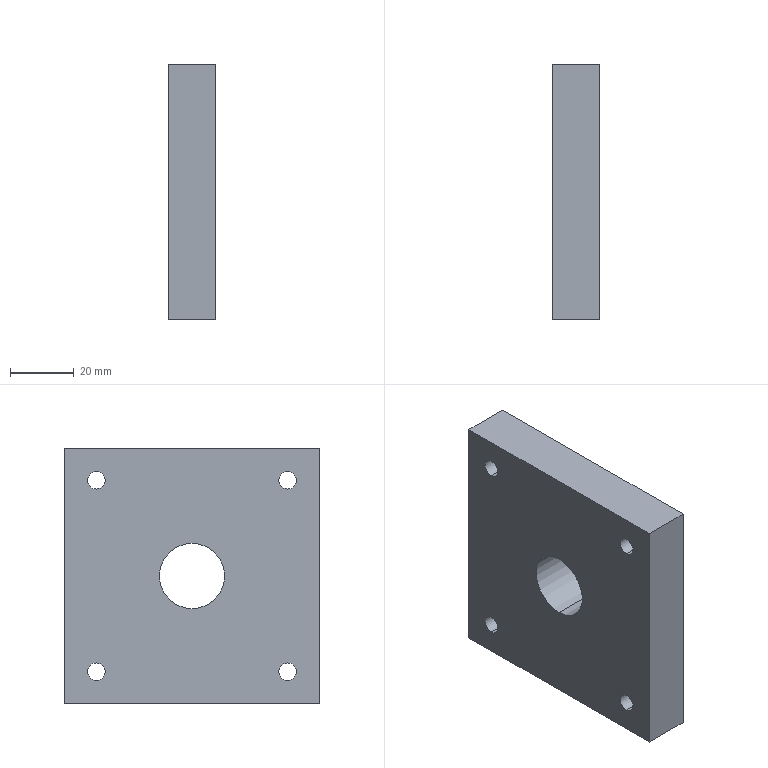Part | STEP file | 09-39 Cylinder top plate | 1 solid | 16 faces | box 15 x 80 x 80 mm | volume 89624 mm3 | cylinder 10 | plane 6 | commonest cylinder face diameters 5.5 x8 20.5 x2
STEP:
#1=CARTESIAN_POINT('',(0.,0.,0.));
#2=DIRECTION('',(0.,0.,1.));
#3=DIRECTION('',(1.,0.,0.));
#4=AXIS2_PLACEMENT_3D('',#1,#2,#3);
#5=CARTESIAN_POINT('',(0.,0.,-10.25));
#6=VERTEX_POINT('',#5);
#7=CARTESIAN_POINT('',(15.,0.,-10.25));
#8=VERTEX_POINT('',#7);
#9=CARTESIAN_POINT('',(0.,0.,-10.25));
#10=DIRECTION('',(1.,0.,0.));
#11=VECTOR('',#10,1.);
#12=LINE('',#9,#11);
#13=CARTESIAN_POINT('',(0.,0.,0.));
#14=DIRECTION('',(1.,0.,0.));
#15=DIRECTION('',(0.,0.,-1.));
#16=AXIS2_PLACEMENT_3D('',#13,#14,#15);
#17=CYLINDRICAL_SURFACE('',#16,10.25);
#18=CARTESIAN_POINT('',(6.283,0.));
#19=DIRECTION('',(0.,1.));
#20=VECTOR('',#19,1.);
#21=LINE('',#18,#20);
#22=(GEOMETRIC_REPRESENTATION_CONTEXT(2)PARAMETRIC_REPRESENTATION_CONTEXT()REPRESENTATION_CONTEXT('',''));
#23=DEFINITIONAL_REPRESENTATION('',(#21),#22);
#24=PCURVE('',#17,#23);
#25=CARTESIAN_POINT('',(0.,0.,0.));
#26=DIRECTION('',(1.,0.,0.));
#27=DIRECTION('',(0.,0.,-1.));
#28=AXIS2_PLACEMENT_3D('',#25,#26,#27);
#29=CYLINDRICAL_SURFACE('',#28,10.25);
#30=CARTESIAN_POINT('',(0.,0.));
#31=DIRECTION('',(0.,1.));
#32=VECTOR('',#31,1.);
#33=LINE('',#30,#32);
#34=(GEOMETRIC_REPRESENTATION_CONTEXT(2)PARAMETRIC_REPRESENTATION_CONTEXT()REPRESENTATION_CONTEXT('',''));
#35=DEFINITIONAL_REPRESENTATION('',(#33),#34);
#36=PCURVE('',#29,#35);
#37=SURFACE_CURVE('',#12,(#24,#36),.PCURVE_S1.);
#38=EDGE_CURVE('',#6,#8,#37,.T.);
#39=ORIENTED_EDGE('',*,*,#38,.T.);
#40=CARTESIAN_POINT('',(15.,0.,10.25));
#41=VERTEX_POINT('',#40);
#42=CARTESIAN_POINT('',(15.,0.,0.));
#43=DIRECTION('',(1.,0.,0.));
#44=DIRECTION('',(0.,0.,-1.));
#45=AXIS2_PLACEMENT_3D('',#42,#43,#44);
#46=CIRCLE('',#45,10.25);
#47=CARTESIAN_POINT('',(0.,15.));
#48=DIRECTION('',(1.,0.));
#49=VECTOR('',#48,1.);
#50=LINE('',#47,#49);
#51=(GEOMETRIC_REPRESENTATION_CONTEXT(2)PARAMETRIC_REPRESENTATION_CONTEXT()REPRESENTATION_CONTEXT('',''));
#52=DEFINITIONAL_REPRESENTATION('',(#50),#51);
#53=PCURVE('',#17,#52);
#54=CARTESIAN_POINT('',(15.,-40.,-40.));
#55=DIRECTION('',(-1.,0.,0.));
#56=DIRECTION('',(0.,0.,1.));
#57=AXIS2_PLACEMENT_3D('',#54,#55,#56);
#58=PLANE('',#57);
#59=CARTESIAN_POINT('',(29.75,40.));
#60=CARTESIAN_POINT('',(29.75,57.754));
#61=CARTESIAN_POINT('',(45.125,48.877));
#62=CARTESIAN_POINT('',(60.5,40.));
#63=CARTESIAN_POINT('',(45.125,31.123));
#64=CARTESIAN_POINT('',(29.75,22.246));
#65=CARTESIAN_POINT('',(29.75,40.));
#66=(BOUNDED_CURVE()B_SPLINE_CURVE(2,(#59,#60,#61,#62,#63,#64,#65),.UNSPECIFIED.,.T.,.F.)B_SPLINE_CURVE_WITH_KNOTS((1,2,2,2,2,1),(-2.094,0.,2.094,4.189,6.283,8.378),.UNSPECIFIED.)CURVE()GEOMETRIC_REPRESENTATION_ITEM()RATIONAL_B_SPLINE_CURVE((1.,0.5,1.,0.5,1.,0.5,1.))REPRESENTATION_ITEM(''));
#67=(GEOMETRIC_REPRESENTATION_CONTEXT(2)PARAMETRIC_REPRESENTATION_CONTEXT()REPRESENTATION_CONTEXT('',''));
#68=DEFINITIONAL_REPRESENTATION('',(#66),#67);
#69=PCURVE('',#58,#68);
#70=SURFACE_CURVE('',#46,(#53,#69),.PCURVE_S1.);
#71=EDGE_CURVE('',#41,#8,#70,.T.);
#72=ORIENTED_EDGE('',*,*,#71,.F.);
#73=CARTESIAN_POINT('',(0.,0.,10.25));
#74=VERTEX_POINT('',#73);
#75=CARTESIAN_POINT('',(0.,0.,10.25));
#76=DIRECTION('',(1.,0.,0.));
#77=VECTOR('',#76,1.);
#78=LINE('',#75,#77);
#79=CARTESIAN_POINT('',(3.142,0.));
#80=DIRECTION('',(0.,1.));
#81=VECTOR('',#80,1.);
#82=LINE('',#79,#81);
#83=(GEOMETRIC_REPRESENTATION_CONTEXT(2)PARAMETRIC_REPRESENTATION_CONTEXT()REPRESENTATION_CONTEXT('',''));
#84=DEFINITIONAL_REPRESENTATION('',(#82),#83);
#85=PCURVE('',#17,#84);
#86=CARTESIAN_POINT('',(3.142,0.));
#87=DIRECTION('',(0.,1.));
#88=VECTOR('',#87,1.);
#89=LINE('',#86,#88);
#90=(GEOMETRIC_REPRESENTATION_CONTEXT(2)PARAMETRIC_REPRESENTATION_CONTEXT()REPRESENTATION_CONTEXT('',''));
#91=DEFINITIONAL_REPRESENTATION('',(#89),#90);
#92=PCURVE('',#29,#91);
#93=SURFACE_CURVE('',#78,(#85,#92),.PCURVE_S1.);
#94=EDGE_CURVE('',#74,#41,#93,.T.);
#95=ORIENTED_EDGE('',*,*,#94,.F.);
#96=CARTESIAN_POINT('',(0.,0.,0.));
#97=DIRECTION('',(-1.,0.,0.));
#98=DIRECTION('',(0.,0.,-1.));
#99=AXIS2_PLACEMENT_3D('',#96,#97,#98);
#100=CIRCLE('',#99,10.25);
#101=CARTESIAN_POINT('',(6.283,0.));
#102=DIRECTION('',(-1.,0.));
#103=VECTOR('',#102,1.);
#104=LINE('',#101,#103);
#105=(GEOMETRIC_REPRESENTATION_CONTEXT(2)PARAMETRIC_REPRESENTATION_CONTEXT()REPRESENTATION_CONTEXT('',''));
#106=DEFINITIONAL_REPRESENTATION('',(#104),#105);
#107=PCURVE('',#17,#106);
#108=CARTESIAN_POINT('',(0.,-40.,-40.));
#109=DIRECTION('',(-1.,0.,0.));
#110=DIRECTION('',(0.,0.,1.));
#111=AXIS2_PLACEMENT_3D('',#108,#109,#110);
#112=PLANE('',#111);
#113=CARTESIAN_POINT('',(40.,40.));
#114=DIRECTION('',(-1.,0.));
#115=AXIS2_PLACEMENT_2D('',#113,#114);
#116=CIRCLE('',#115,10.25);
#117=(GEOMETRIC_REPRESENTATION_CONTEXT(2)PARAMETRIC_REPRESENTATION_CONTEXT()REPRESENTATION_CONTEXT('',''));
#118=DEFINITIONAL_REPRESENTATION('',(#116),#117);
#119=PCURVE('',#112,#118);
#120=SURFACE_CURVE('',#100,(#107,#119),.PCURVE_S1.);
#121=EDGE_CURVE('',#6,#74,#120,.T.);
#122=ORIENTED_EDGE('',*,*,#121,.F.);
#123=EDGE_LOOP('',(#39,#72,#95,#122));
#124=FACE_BOUND('',#123,.F.);
#125=ADVANCED_FACE('',(#124),#17,.F.);
#126=CARTESIAN_POINT('',(0.,30.,27.25));
#127=VERTEX_POINT('',#126);
#128=CARTESIAN_POINT('',(15.,30.,27.25));
#129=VERTEX_POINT('',#128);
#130=CARTESIAN_POINT('',(0.,30.,27.25));
#131=DIRECTION('',(1.,0.,0.));
#132=VECTOR('',#131,1.);
#133=LINE('',#130,#132);
#134=CARTESIAN_POINT('',(0.,30.,30.));
#135=DIRECTION('',(1.,0.,0.));
#136=DIRECTION('',(0.,0.,-1.));
#137=AXIS2_PLACEMENT_3D('',#134,#135,#136);
#138=CYLINDRICAL_SURFACE('',#137,2.75);
#139=CARTESIAN_POINT('',(6.283,0.));
#140=DIRECTION('',(0.,1.));
#141=VECTOR('',#140,1.);
#142=LINE('',#139,#141);
#143=(GEOMETRIC_REPRESENTATION_CONTEXT(2)PARAMETRIC_REPRESENTATION_CONTEXT()REPRESENTATION_CONTEXT('',''));
#144=DEFINITIONAL_REPRESENTATION('',(#142),#143);
#145=PCURVE('',#138,#144);
#146=CARTESIAN_POINT('',(0.,30.,30.));
#147=DIRECTION('',(1.,0.,0.));
#148=DIRECTION('',(0.,0.,-1.));
#149=AXIS2_PLACEMENT_3D('',#146,#147,#148);
#150=CYLINDRICAL_SURFACE('',#149,2.75);
#151=CARTESIAN_POINT('',(0.,0.));
#152=DIRECTION('',(0.,1.));
#153=VECTOR('',#152,1.);
#154=LINE('',#151,#153);
#155=(GEOMETRIC_REPRESENTATION_CONTEXT(2)PARAMETRIC_REPRESENTATION_CONTEXT()REPRESENTATION_CONTEXT('',''));
#156=DEFINITIONAL_REPRESENTATION('',(#154),#155);
#157=PCURVE('',#150,#156);
#158=SURFACE_CURVE('',#133,(#145,#157),.PCURVE_S1.);
#159=EDGE_CURVE('',#127,#129,#158,.T.);
#160=ORIENTED_EDGE('',*,*,#159,.T.);
#161=CARTESIAN_POINT('',(15.,30.,32.75));
#162=VERTEX_POINT('',#161);
#163=CARTESIAN_POINT('',(15.,30.,30.));
#164=DIRECTION('',(1.,0.,0.));
#165=DIRECTION('',(0.,0.,-1.));
#166=AXIS2_PLACEMENT_3D('',#163,#164,#165);
#167=CIRCLE('',#166,2.75);
#168=CARTESIAN_POINT('',(0.,15.));
#169=DIRECTION('',(1.,0.));
#170=VECTOR('',#169,1.);
#171=LINE('',#168,#170);
#172=(GEOMETRIC_REPRESENTATION_CONTEXT(2)PARAMETRIC_REPRESENTATION_CONTEXT()REPRESENTATION_CONTEXT('',''));
#173=DEFINITIONAL_REPRESENTATION('',(#171),#172);
#174=PCURVE('',#138,#173);
#175=CARTESIAN_POINT('',(67.25,70.));
#176=CARTESIAN_POINT('',(67.25,74.763));
#177=CARTESIAN_POINT('',(71.375,72.382));
#178=CARTESIAN_POINT('',(75.5,70.));
#179=CARTESIAN_POINT('',(71.375,67.618));
#180=CARTESIAN_POINT('',(67.25,65.237));
#181=CARTESIAN_POINT('',(67.25,70.));
#182=(BOUNDED_CURVE()B_SPLINE_CURVE(2,(#175,#176,#177,#178,#179,#180,#181),.UNSPECIFIED.,.T.,.F.)B_SPLINE_CURVE_WITH_KNOTS((1,2,2,2,2,1),(-2.094,0.,2.094,4.189,6.283,8.378),.UNSPECIFIED.)CURVE()GEOMETRIC_REPRESENTATION_ITEM()RATIONAL_B_SPLINE_CURVE((1.,0.5,1.,0.5,1.,0.5,1.))REPRESENTATION_ITEM(''));
#183=(GEOMETRIC_REPRESENTATION_CONTEXT(2)PARAMETRIC_REPRESENTATION_CONTEXT()REPRESENTATION_CONTEXT('',''));
#184=DEFINITIONAL_REPRESENTATION('',(#182),#183);
#185=PCURVE('',#58,#184);
#186=SURFACE_CURVE('',#167,(#174,#185),.PCURVE_S1.);
#187=EDGE_CURVE('',#162,#129,#186,.T.);
#188=ORIENTED_EDGE('',*,*,#187,.F.);
#189=CARTESIAN_POINT('',(0.,30.,32.75));
#190=VERTEX_POINT('',#189);
#191=CARTESIAN_POINT('',(0.,30.,32.75));
#192=DIRECTION('',(1.,0.,0.));
#193=VECTOR('',#192,1.);
#194=LINE('',#191,#193);
#195=CARTESIAN_POINT('',(3.142,0.));
#196=DIRECTION('',(0.,1.));
#197=VECTOR('',#196,1.);
#198=LINE('',#195,#197);
#199=(GEOMETRIC_REPRESENTATION_CONTEXT(2)PARAMETRIC_REPRESENTATION_CONTEXT()REPRESENTATION_CONTEXT('',''));
#200=DEFINITIONAL_REPRESENTATION('',(#198),#199);
#201=PCURVE('',#138,#200);
#202=CARTESIAN_POINT('',(3.142,0.));
#203=DIRECTION('',(0.,1.));
#204=VECTOR('',#203,1.);
#205=LINE('',#202,#204);
#206=(GEOMETRIC_REPRESENTATION_CONTEXT(2)PARAMETRIC_REPRESENTATION_CONTEXT()REPRESENTATION_CONTEXT('',''));
#207=DEFINITIONAL_REPRESENTATION('',(#205),#206);
#208=PCURVE('',#150,#207);
#209=SURFACE_CURVE('',#194,(#201,#208),.PCURVE_S1.);
#210=EDGE_CURVE('',#190,#162,#209,.T.);
#211=ORIENTED_EDGE('',*,*,#210,.F.);
#212=CARTESIAN_POINT('',(0.,30.,30.));
#213=DIRECTION('',(1.,0.,0.));
#214=DIRECTION('',(0.,0.,-1.));
#215=AXIS2_PLACEMENT_3D('',#212,#213,#214);
#216=CIRCLE('',#215,2.75);
#217=CARTESIAN_POINT('',(0.,0.));
#218=DIRECTION('',(1.,0.));
#219=VECTOR('',#218,1.);
#220=LINE('',#217,#219);
#221=(GEOMETRIC_REPRESENTATION_CONTEXT(2)PARAMETRIC_REPRESENTATION_CONTEXT()REPRESENTATION_CONTEXT('',''));
#222=DEFINITIONAL_REPRESENTATION('',(#220),#221);
#223=PCURVE('',#138,#222);
#224=CARTESIAN_POINT('',(67.25,70.));
#225=CARTESIAN_POINT('',(67.25,74.763));
#226=CARTESIAN_POINT('',(71.375,72.382));
#227=CARTESIAN_POINT('',(75.5,70.));
#228=CARTESIAN_POINT('',(71.375,67.618));
#229=CARTESIAN_POINT('',(67.25,65.237));
#230=CARTESIAN_POINT('',(67.25,70.));
#231=(BOUNDED_CURVE()B_SPLINE_CURVE(2,(#224,#225,#226,#227,#228,#229,#230),.UNSPECIFIED.,.T.,.F.)B_SPLINE_CURVE_WITH_KNOTS((1,2,2,2,2,1),(-2.094,0.,2.094,4.189,6.283,8.378),.UNSPECIFIED.)CURVE()GEOMETRIC_REPRESENTATION_ITEM()RATIONAL_B_SPLINE_CURVE((1.,0.5,1.,0.5,1.,0.5,1.))REPRESENTATION_ITEM(''));
#232=(GEOMETRIC_REPRESENTATION_CONTEXT(2)PARAMETRIC_REPRESENTATION_CONTEXT()REPRESENTATION_CONTEXT('',''));
#233=DEFINITIONAL_REPRESENTATION('',(#231),#232);
#234=PCURVE('',#112,#233);
#235=SURFACE_CURVE('',#216,(#223,#234),.PCURVE_S1.);
#236=EDGE_CURVE('',#190,#127,#235,.T.);
#237=ORIENTED_EDGE('',*,*,#236,.T.);
#238=EDGE_LOOP('',(#160,#188,#211,#237));
#239=FACE_BOUND('',#238,.F.);
#240=ADVANCED_FACE('',(#239),#138,.F.);
#241=CARTESIAN_POINT('',(0.,30.,-32.75));
#242=VERTEX_POINT('',#241);
#243=CARTESIAN_POINT('',(15.,30.,-32.75));
#244=VERTEX_POINT('',#243);
#245=CARTESIAN_POINT('',(0.,30.,-32.75));
#246=DIRECTION('',(1.,0.,0.));
#247=VECTOR('',#246,1.);
#248=LINE('',#245,#247);
#249=CARTESIAN_POINT('',(0.,30.,-30.));
#250=DIRECTION('',(1.,0.,0.));
#251=DIRECTION('',(0.,0.,-1.));
#252=AXIS2_PLACEMENT_3D('',#249,#250,#251);
#253=CYLINDRICAL_SURFACE('',#252,2.75);
#254=CARTESIAN_POINT('',(6.283,0.));
#255=DIRECTION('',(0.,1.));
#256=VECTOR('',#255,1.);
#257=LINE('',#254,#256);
#258=(GEOMETRIC_REPRESENTATION_CONTEXT(2)PARAMETRIC_REPRESENTATION_CONTEXT()REPRESENTATION_CONTEXT('',''));
#259=DEFINITIONAL_REPRESENTATION('',(#257),#258);
#260=PCURVE('',#253,#259);
#261=CARTESIAN_POINT('',(0.,30.,-30.));
#262=DIRECTION('',(1.,0.,0.));
#263=DIRECTION('',(0.,0.,-1.));
#264=AXIS2_PLACEMENT_3D('',#261,#262,#263);
#265=CYLINDRICAL_SURFACE('',#264,2.75);
#266=CARTESIAN_POINT('',(0.,0.));
#267=DIRECTION('',(0.,1.));
#268=VECTOR('',#267,1.);
#269=LINE('',#266,#268);
#270=(GEOMETRIC_REPRESENTATION_CONTEXT(2)PARAMETRIC_REPRESENTATION_CONTEXT()REPRESENTATION_CONTEXT('',''));
#271=DEFINITIONAL_REPRESENTATION('',(#269),#270);
#272=PCURVE('',#265,#271);
#273=SURFACE_CURVE('',#248,(#260,#272),.PCURVE_S1.);
#274=EDGE_CURVE('',#242,#244,#273,.T.);
#275=ORIENTED_EDGE('',*,*,#274,.T.);
#276=CARTESIAN_POINT('',(15.,30.,-27.25));
#277=VERTEX_POINT('',#276);
#278=CARTESIAN_POINT('',(15.,30.,-30.));
#279=DIRECTION('',(1.,0.,0.));
#280=DIRECTION('',(0.,0.,-1.));
#281=AXIS2_PLACEMENT_3D('',#278,#279,#280);
#282=CIRCLE('',#281,2.75);
#283=CARTESIAN_POINT('',(0.,15.));
#284=DIRECTION('',(1.,0.));
#285=VECTOR('',#284,1.);
#286=LINE('',#283,#285);
#287=(GEOMETRIC_REPRESENTATION_CONTEXT(2)PARAMETRIC_REPRESENTATION_CONTEXT()REPRESENTATION_CONTEXT('',''));
#288=DEFINITIONAL_REPRESENTATION('',(#286),#287);
#289=PCURVE('',#253,#288);
#290=CARTESIAN_POINT('',(7.25,70.));
#291=CARTESIAN_POINT('',(7.25,74.763));
#292=CARTESIAN_POINT('',(11.375,72.382));
#293=CARTESIAN_POINT('',(15.5,70.));
#294=CARTESIAN_POINT('',(11.375,67.618));
#295=CARTESIAN_POINT('',(7.25,65.237));
#296=CARTESIAN_POINT('',(7.25,70.));
#297=(BOUNDED_CURVE()B_SPLINE_CURVE(2,(#290,#291,#292,#293,#294,#295,#296),.UNSPECIFIED.,.T.,.F.)B_SPLINE_CURVE_WITH_KNOTS((1,2,2,2,2,1),(-2.094,0.,2.094,4.189,6.283,8.378),.UNSPECIFIED.)CURVE()GEOMETRIC_REPRESENTATION_ITEM()RATIONAL_B_SPLINE_CURVE((1.,0.5,1.,0.5,1.,0.5,1.))REPRESENTATION_ITEM(''));
#298=(GEOMETRIC_REPRESENTATION_CONTEXT(2)PARAMETRIC_REPRESENTATION_CONTEXT()REPRESENTATION_CONTEXT('',''));
#299=DEFINITIONAL_REPRESENTATION('',(#297),#298);
#300=PCURVE('',#58,#299);
#301=SURFACE_CURVE('',#282,(#289,#300),.PCURVE_S1.);
#302=EDGE_CURVE('',#277,#244,#301,.T.);
#303=ORIENTED_EDGE('',*,*,#302,.F.);
#304=CARTESIAN_POINT('',(0.,30.,-27.25));
#305=VERTEX_POINT('',#304);
#306=CARTESIAN_POINT('',(0.,30.,-27.25));
#307=DIRECTION('',(1.,0.,0.));
#308=VECTOR('',#307,1.);
#309=LINE('',#306,#308);
#310=CARTESIAN_POINT('',(3.142,0.));
#311=DIRECTION('',(0.,1.));
#312=VECTOR('',#311,1.);
#313=LINE('',#310,#312);
#314=(GEOMETRIC_REPRESENTATION_CONTEXT(2)PARAMETRIC_REPRESENTATION_CONTEXT()REPRESENTATION_CONTEXT('',''));
#315=DEFINITIONAL_REPRESENTATION('',(#313),#314);
#316=PCURVE('',#253,#315);
#317=CARTESIAN_POINT('',(3.142,0.));
#318=DIRECTION('',(0.,1.));
#319=VECTOR('',#318,1.);
#320=LINE('',#317,#319);
#321=(GEOMETRIC_REPRESENTATION_CONTEXT(2)PARAMETRIC_REPRESENTATION_CONTEXT()REPRESENTATION_CONTEXT('',''));
#322=DEFINITIONAL_REPRESENTATION('',(#320),#321);
#323=PCURVE('',#265,#322);
#324=SURFACE_CURVE('',#309,(#316,#323),.PCURVE_S1.);
#325=EDGE_CURVE('',#305,#277,#324,.T.);
#326=ORIENTED_EDGE('',*,*,#325,.F.);
#327=CARTESIAN_POINT('',(0.,30.,-30.));
#328=DIRECTION('',(1.,0.,0.));
#329=DIRECTION('',(0.,0.,-1.));
#330=AXIS2_PLACEMENT_3D('',#327,#328,#329);
#331=CIRCLE('',#330,2.75);
#332=CARTESIAN_POINT('',(0.,0.));
#333=DIRECTION('',(1.,0.));
#334=VECTOR('',#333,1.);
#335=LINE('',#332,#334);
#336=(GEOMETRIC_REPRESENTATION_CONTEXT(2)PARAMETRIC_REPRESENTATION_CONTEXT()REPRESENTATION_CONTEXT('',''));
#337=DEFINITIONAL_REPRESENTATION('',(#335),#336);
#338=PCURVE('',#253,#337);
#339=CARTESIAN_POINT('',(7.25,70.));
#340=CARTESIAN_POINT('',(7.25,74.763));
#341=CARTESIAN_POINT('',(11.375,72.382));
#342=CARTESIAN_POINT('',(15.5,70.));
#343=CARTESIAN_POINT('',(11.375,67.618));
#344=CARTESIAN_POINT('',(7.25,65.237));
#345=CARTESIAN_POINT('',(7.25,70.));
#346=(BOUNDED_CURVE()B_SPLINE_CURVE(2,(#339,#340,#341,#342,#343,#344,#345),.UNSPECIFIED.,.T.,.F.)B_SPLINE_CURVE_WITH_KNOTS((1,2,2,2,2,1),(-2.094,0.,2.094,4.189,6.283,8.378),.UNSPECIFIED.)CURVE()GEOMETRIC_REPRESENTATION_ITEM()RATIONAL_B_SPLINE_CURVE((1.,0.5,1.,0.5,1.,0.5,1.))REPRESENTATION_ITEM(''));
#347=(GEOMETRIC_REPRESENTATION_CONTEXT(2)PARAMETRIC_REPRESENTATION_CONTEXT()REPRESENTATION_CONTEXT('',''));
#348=DEFINITIONAL_REPRESENTATION('',(#346),#347);
#349=PCURVE('',#112,#348);
#350=SURFACE_CURVE('',#331,(#338,#349),.PCURVE_S1.);
#351=EDGE_CURVE('',#305,#242,#350,.T.);
#352=ORIENTED_EDGE('',*,*,#351,.T.);
#353=EDGE_LOOP('',(#275,#303,#326,#352));
#354=FACE_BOUND('',#353,.F.);
#355=ADVANCED_FACE('',(#354),#253,.F.);
#356=CARTESIAN_POINT('',(0.,-30.,-32.75));
#357=VERTEX_POINT('',#356);
#358=CARTESIAN_POINT('',(15.,-30.,-32.75));
#359=VERTEX_POINT('',#358);
#360=CARTESIAN_POINT('',(0.,-30.,-32.75));
#361=DIRECTION('',(1.,0.,0.));
#362=VECTOR('',#361,1.);
#363=LINE('',#360,#362);
#364=CARTESIAN_POINT('',(0.,-30.,-30.));
#365=DIRECTION('',(1.,0.,0.));
#366=DIRECTION('',(0.,0.,-1.));
#367=AXIS2_PLACEMENT_3D('',#364,#365,#366);
#368=CYLINDRICAL_SURFACE('',#367,2.75);
#369=CARTESIAN_POINT('',(6.283,0.));
#370=DIRECTION('',(0.,1.));
#371=VECTOR('',#370,1.);
#372=LINE('',#369,#371);
#373=(GEOMETRIC_REPRESENTATION_CONTEXT(2)PARAMETRIC_REPRESENTATION_CONTEXT()REPRESENTATION_CONTEXT('',''));
#374=DEFINITIONAL_REPRESENTATION('',(#372),#373);
#375=PCURVE('',#368,#374);
#376=CARTESIAN_POINT('',(0.,-30.,-30.));
#377=DIRECTION('',(1.,0.,0.));
#378=DIRECTION('',(0.,0.,-1.));
#379=AXIS2_PLACEMENT_3D('',#376,#377,#378);
#380=CYLINDRICAL_SURFACE('',#379,2.75);
#381=CARTESIAN_POINT('',(0.,0.));
#382=DIRECTION('',(0.,1.));
#383=VECTOR('',#382,1.);
#384=LINE('',#381,#383);
#385=(GEOMETRIC_REPRESENTATION_CONTEXT(2)PARAMETRIC_REPRESENTATION_CONTEXT()REPRESENTATION_CONTEXT('',''));
#386=DEFINITIONAL_REPRESENTATION('',(#384),#385);
#387=PCURVE('',#380,#386);
#388=SURFACE_CURVE('',#363,(#375,#387),.PCURVE_S1.);
#389=EDGE_CURVE('',#357,#359,#388,.T.);
#390=ORIENTED_EDGE('',*,*,#389,.T.);
#391=CARTESIAN_POINT('',(15.,-30.,-27.25));
#392=VERTEX_POINT('',#391);
#393=CARTESIAN_POINT('',(15.,-30.,-30.));
#394=DIRECTION('',(1.,0.,0.));
#395=DIRECTION('',(0.,0.,-1.));
#396=AXIS2_PLACEMENT_3D('',#393,#394,#395);
#397=CIRCLE('',#396,2.75);
#398=CARTESIAN_POINT('',(0.,15.));
#399=DIRECTION('',(1.,0.));
#400=VECTOR('',#399,1.);
#401=LINE('',#398,#400);
#402=(GEOMETRIC_REPRESENTATION_CONTEXT(2)PARAMETRIC_REPRESENTATION_CONTEXT()REPRESENTATION_CONTEXT('',''));
#403=DEFINITIONAL_REPRESENTATION('',(#401),#402);
#404=PCURVE('',#368,#403);
#405=CARTESIAN_POINT('',(7.25,10.));
#406=CARTESIAN_POINT('',(7.25,14.763));
#407=CARTESIAN_POINT('',(11.375,12.382));
#408=CARTESIAN_POINT('',(15.5,10.));
#409=CARTESIAN_POINT('',(11.375,7.618));
#410=CARTESIAN_POINT('',(7.25,5.237));
#411=CARTESIAN_POINT('',(7.25,10.));
#412=(BOUNDED_CURVE()B_SPLINE_CURVE(2,(#405,#406,#407,#408,#409,#410,#411),.UNSPECIFIED.,.T.,.F.)B_SPLINE_CURVE_WITH_KNOTS((1,2,2,2,2,1),(-2.094,0.,2.094,4.189,6.283,8.378),.UNSPECIFIED.)CURVE()GEOMETRIC_REPRESENTATION_ITEM()RATIONAL_B_SPLINE_CURVE((1.,0.5,1.,0.5,1.,0.5,1.))REPRESENTATION_ITEM(''));
#413=(GEOMETRIC_REPRESENTATION_CONTEXT(2)PARAMETRIC_REPRESENTATION_CONTEXT()REPRESENTATION_CONTEXT('',''));
#414=DEFINITIONAL_REPRESENTATION('',(#412),#413);
#415=PCURVE('',#58,#414);
#416=SURFACE_CURVE('',#397,(#404,#415),.PCURVE_S1.);
#417=EDGE_CURVE('',#392,#359,#416,.T.);
#418=ORIENTED_EDGE('',*,*,#417,.F.);
#419=CARTESIAN_POINT('',(0.,-30.,-27.25));
#420=VERTEX_POINT('',#419);
#421=CARTESIAN_POINT('',(0.,-30.,-27.25));
#422=DIRECTION('',(1.,0.,0.));
#423=VECTOR('',#422,1.);
#424=LINE('',#421,#423);
#425=CARTESIAN_POINT('',(3.142,0.));
#426=DIRECTION('',(0.,1.));
#427=VECTOR('',#426,1.);
#428=LINE('',#425,#427);
#429=(GEOMETRIC_REPRESENTATION_CONTEXT(2)PARAMETRIC_REPRESENTATION_CONTEXT()REPRESENTATION_CONTEXT('',''));
#430=DEFINITIONAL_REPRESENTATION('',(#428),#429);
#431=PCURVE('',#368,#430);
#432=CARTESIAN_POINT('',(3.142,0.));
#433=DIRECTION('',(0.,1.));
#434=VECTOR('',#433,1.);
#435=LINE('',#432,#434);
#436=(GEOMETRIC_REPRESENTATION_CONTEXT(2)PARAMETRIC_REPRESENTATION_CONTEXT()REPRESENTATION_CONTEXT('',''));
#437=DEFINITIONAL_REPRESENTATION('',(#435),#436);
#438=PCURVE('',#380,#437);
#439=SURFACE_CURVE('',#424,(#431,#438),.PCURVE_S1.);
#440=EDGE_CURVE('',#420,#392,#439,.T.);
#441=ORIENTED_EDGE('',*,*,#440,.F.);
#442=CARTESIAN_POINT('',(0.,-30.,-30.));
#443=DIRECTION('',(1.,0.,0.));
#444=DIRECTION('',(0.,0.,-1.));
#445=AXIS2_PLACEMENT_3D('',#442,#443,#444);
#446=CIRCLE('',#445,2.75);
#447=CARTESIAN_POINT('',(0.,0.));
#448=DIRECTION('',(1.,0.));
#449=VECTOR('',#448,1.);
#450=LINE('',#447,#449);
#451=(GEOMETRIC_REPRESENTATION_CONTEXT(2)PARAMETRIC_REPRESENTATION_CONTEXT()REPRESENTATION_CONTEXT('',''));
#452=DEFINITIONAL_REPRESENTATION('',(#450),#451);
#453=PCURVE('',#368,#452);
#454=CARTESIAN_POINT('',(7.25,10.));
#455=CARTESIAN_POINT('',(7.25,14.763));
#456=CARTESIAN_POINT('',(11.375,12.382));
#457=CARTESIAN_POINT('',(15.5,10.));
#458=CARTESIAN_POINT('',(11.375,7.618));
#459=CARTESIAN_POINT('',(7.25,5.237));
#460=CARTESIAN_POINT('',(7.25,10.));
#461=(BOUNDED_CURVE()B_SPLINE_CURVE(2,(#454,#455,#456,#457,#458,#459,#460),.UNSPECIFIED.,.T.,.F.)B_SPLINE_CURVE_WITH_KNOTS((1,2,2,2,2,1),(-2.094,0.,2.094,4.189,6.283,8.378),.UNSPECIFIED.)CURVE()GEOMETRIC_REPRESENTATION_ITEM()RATIONAL_B_SPLINE_CURVE((1.,0.5,1.,0.5,1.,0.5,1.))REPRESENTATION_ITEM(''));
#462=(GEOMETRIC_REPRESENTATION_CONTEXT(2)PARAMETRIC_REPRESENTATION_CONTEXT()REPRESENTATION_CONTEXT('',''));
#463=DEFINITIONAL_REPRESENTATION('',(#461),#462);
#464=PCURVE('',#112,#463);
#465=SURFACE_CURVE('',#446,(#453,#464),.PCURVE_S1.);
#466=EDGE_CURVE('',#420,#357,#465,.T.);
#467=ORIENTED_EDGE('',*,*,#466,.T.);
#468=EDGE_LOOP('',(#390,#418,#441,#467));
#469=FACE_BOUND('',#468,.F.);
#470=ADVANCED_FACE('',(#469),#368,.F.);
#471=CARTESIAN_POINT('',(0.,-30.,27.25));
#472=VERTEX_POINT('',#471);
#473=CARTESIAN_POINT('',(15.,-30.,27.25));
#474=VERTEX_POINT('',#473);
#475=CARTESIAN_POINT('',(0.,-30.,27.25));
#476=DIRECTION('',(1.,0.,0.));
#477=VECTOR('',#476,1.);
#478=LINE('',#475,#477);
#479=CARTESIAN_POINT('',(0.,-30.,30.));
#480=DIRECTION('',(1.,0.,0.));
#481=DIRECTION('',(0.,0.,-1.));
#482=AXIS2_PLACEMENT_3D('',#479,#480,#481);
#483=CYLINDRICAL_SURFACE('',#482,2.75);
#484=CARTESIAN_POINT('',(6.283,0.));
#485=DIRECTION('',(0.,1.));
#486=VECTOR('',#485,1.);
#487=LINE('',#484,#486);
#488=(GEOMETRIC_REPRESENTATION_CONTEXT(2)PARAMETRIC_REPRESENTATION_CONTEXT()REPRESENTATION_CONTEXT('',''));
#489=DEFINITIONAL_REPRESENTATION('',(#487),#488);
#490=PCURVE('',#483,#489);
#491=CARTESIAN_POINT('',(0.,-30.,30.));
#492=DIRECTION('',(1.,0.,0.));
#493=DIRECTION('',(0.,0.,-1.));
#494=AXIS2_PLACEMENT_3D('',#491,#492,#493);
#495=CYLINDRICAL_SURFACE('',#494,2.75);
#496=CARTESIAN_POINT('',(0.,0.));
#497=DIRECTION('',(0.,1.));
#498=VECTOR('',#497,1.);
#499=LINE('',#496,#498);
#500=(GEOMETRIC_REPRESENTATION_CONTEXT(2)PARAMETRIC_REPRESENTATION_CONTEXT()REPRESENTATION_CONTEXT('',''));
#501=DEFINITIONAL_REPRESENTATION('',(#499),#500);
#502=PCURVE('',#495,#501);
#503=SURFACE_CURVE('',#478,(#490,#502),.PCURVE_S1.);
#504=EDGE_CURVE('',#472,#474,#503,.T.);
#505=ORIENTED_EDGE('',*,*,#504,.T.);
#506=CARTESIAN_POINT('',(15.,-30.,32.75));
#507=VERTEX_POINT('',#506);
#508=CARTESIAN_POINT('',(15.,-30.,30.));
#509=DIRECTION('',(1.,0.,0.));
#510=DIRECTION('',(0.,0.,-1.));
#511=AXIS2_PLACEMENT_3D('',#508,#509,#510);
#512=CIRCLE('',#511,2.75);
#513=CARTESIAN_POINT('',(0.,15.));
#514=DIRECTION('',(1.,0.));
#515=VECTOR('',#514,1.);
#516=LINE('',#513,#515);
#517=(GEOMETRIC_REPRESENTATION_CONTEXT(2)PARAMETRIC_REPRESENTATION_CONTEXT()REPRESENTATION_CONTEXT('',''));
#518=DEFINITIONAL_REPRESENTATION('',(#516),#517);
#519=PCURVE('',#483,#518);
#520=CARTESIAN_POINT('',(67.25,10.));
#521=CARTESIAN_POINT('',(67.25,14.763));
#522=CARTESIAN_POINT('',(71.375,12.382));
#523=CARTESIAN_POINT('',(75.5,10.));
#524=CARTESIAN_POINT('',(71.375,7.618));
#525=CARTESIAN_POINT('',(67.25,5.237));
#526=CARTESIAN_POINT('',(67.25,10.));
#527=(BOUNDED_CURVE()B_SPLINE_CURVE(2,(#520,#521,#522,#523,#524,#525,#526),.UNSPECIFIED.,.T.,.F.)B_SPLINE_CURVE_WITH_KNOTS((1,2,2,2,2,1),(-2.094,0.,2.094,4.189,6.283,8.378),.UNSPECIFIED.)CURVE()GEOMETRIC_REPRESENTATION_ITEM()RATIONAL_B_SPLINE_CURVE((1.,0.5,1.,0.5,1.,0.5,1.))REPRESENTATION_ITEM(''));
#528=(GEOMETRIC_REPRESENTATION_CONTEXT(2)PARAMETRIC_REPRESENTATION_CONTEXT()REPRESENTATION_CONTEXT('',''));
#529=DEFINITIONAL_REPRESENTATION('',(#527),#528);
#530=PCURVE('',#58,#529);
#531=SURFACE_CURVE('',#512,(#519,#530),.PCURVE_S1.);
#532=EDGE_CURVE('',#507,#474,#531,.T.);
#533=ORIENTED_EDGE('',*,*,#532,.F.);
#534=CARTESIAN_POINT('',(0.,-30.,32.75));
#535=VERTEX_POINT('',#534);
#536=CARTESIAN_POINT('',(0.,-30.,32.75));
#537=DIRECTION('',(1.,0.,0.));
#538=VECTOR('',#537,1.);
#539=LINE('',#536,#538);
#540=CARTESIAN_POINT('',(3.142,0.));
#541=DIRECTION('',(0.,1.));
#542=VECTOR('',#541,1.);
#543=LINE('',#540,#542);
#544=(GEOMETRIC_REPRESENTATION_CONTEXT(2)PARAMETRIC_REPRESENTATION_CONTEXT()REPRESENTATION_CONTEXT('',''));
#545=DEFINITIONAL_REPRESENTATION('',(#543),#544);
#546=PCURVE('',#483,#545);
#547=CARTESIAN_POINT('',(3.142,0.));
#548=DIRECTION('',(0.,1.));
#549=VECTOR('',#548,1.);
#550=LINE('',#547,#549);
#551=(GEOMETRIC_REPRESENTATION_CONTEXT(2)PARAMETRIC_REPRESENTATION_CONTEXT()REPRESENTATION_CONTEXT('',''));
#552=DEFINITIONAL_REPRESENTATION('',(#550),#551);
#553=PCURVE('',#495,#552);
#554=SURFACE_CURVE('',#539,(#546,#553),.PCURVE_S1.);
#555=EDGE_CURVE('',#535,#507,#554,.T.);
#556=ORIENTED_EDGE('',*,*,#555,.F.);
#557=CARTESIAN_POINT('',(0.,-30.,30.));
#558=DIRECTION('',(1.,0.,0.));
#559=DIRECTION('',(0.,0.,-1.));
#560=AXIS2_PLACEMENT_3D('',#557,#558,#559);
#561=CIRCLE('',#560,2.75);
#562=CARTESIAN_POINT('',(0.,0.));
#563=DIRECTION('',(1.,0.));
#564=VECTOR('',#563,1.);
#565=LINE('',#562,#564);
#566=(GEOMETRIC_REPRESENTATION_CONTEXT(2)PARAMETRIC_REPRESENTATION_CONTEXT()REPRESENTATION_CONTEXT('',''));
#567=DEFINITIONAL_REPRESENTATION('',(#565),#566);
#568=PCURVE('',#483,#567);
#569=CARTESIAN_POINT('',(67.25,10.));
#570=CARTESIAN_POINT('',(67.25,14.763));
#571=CARTESIAN_POINT('',(71.375,12.382));
#572=CARTESIAN_POINT('',(75.5,10.));
#573=CARTESIAN_POINT('',(71.375,7.618));
#574=CARTESIAN_POINT('',(67.25,5.237));
#575=CARTESIAN_POINT('',(67.25,10.));
#576=(BOUNDED_CURVE()B_SPLINE_CURVE(2,(#569,#570,#571,#572,#573,#574,#575),.UNSPECIFIED.,.T.,.F.)B_SPLINE_CURVE_WITH_KNOTS((1,2,2,2,2,1),(-2.094,0.,2.094,4.189,6.283,8.378),.UNSPECIFIED.)CURVE()GEOMETRIC_REPRESENTATION_ITEM()RATIONAL_B_SPLINE_CURVE((1.,0.5,1.,0.5,1.,0.5,1.))REPRESENTATION_ITEM(''));
#577=(GEOMETRIC_REPRESENTATION_CONTEXT(2)PARAMETRIC_REPRESENTATION_CONTEXT()REPRESENTATION_CONTEXT('',''));
#578=DEFINITIONAL_REPRESENTATION('',(#576),#577);
#579=PCURVE('',#112,#578);
#580=SURFACE_CURVE('',#561,(#568,#579),.PCURVE_S1.);
#581=EDGE_CURVE('',#535,#472,#580,.T.);
#582=ORIENTED_EDGE('',*,*,#581,.T.);
#583=EDGE_LOOP('',(#505,#533,#556,#582));
#584=FACE_BOUND('',#583,.F.);
#585=ADVANCED_FACE('',(#584),#483,.F.);
#586=CARTESIAN_POINT('',(15.,0.,0.));
#587=DIRECTION('',(1.,0.,0.));
#588=DIRECTION('',(0.,0.,-1.));
#589=AXIS2_PLACEMENT_3D('',#586,#587,#588);
#590=CIRCLE('',#589,10.25);
#591=CARTESIAN_POINT('',(0.,15.));
#592=DIRECTION('',(1.,0.));
#593=VECTOR('',#592,1.);
#594=LINE('',#591,#593);
#595=(GEOMETRIC_REPRESENTATION_CONTEXT(2)PARAMETRIC_REPRESENTATION_CONTEXT()REPRESENTATION_CONTEXT('',''));
#596=DEFINITIONAL_REPRESENTATION('',(#594),#595);
#597=PCURVE('',#29,#596);
#598=CARTESIAN_POINT('',(29.75,40.));
#599=CARTESIAN_POINT('',(29.75,57.754));
#600=CARTESIAN_POINT('',(45.125,48.877));
#601=CARTESIAN_POINT('',(60.5,40.));
#602=CARTESIAN_POINT('',(45.125,31.123));
#603=CARTESIAN_POINT('',(29.75,22.246));
#604=CARTESIAN_POINT('',(29.75,40.));
#605=(BOUNDED_CURVE()B_SPLINE_CURVE(2,(#598,#599,#600,#601,#602,#603,#604),.UNSPECIFIED.,.T.,.F.)B_SPLINE_CURVE_WITH_KNOTS((1,2,2,2,2,1),(-2.094,0.,2.094,4.189,6.283,8.378),.UNSPECIFIED.)CURVE()GEOMETRIC_REPRESENTATION_ITEM()RATIONAL_B_SPLINE_CURVE((1.,0.5,1.,0.5,1.,0.5,1.))REPRESENTATION_ITEM(''));
#606=(GEOMETRIC_REPRESENTATION_CONTEXT(2)PARAMETRIC_REPRESENTATION_CONTEXT()REPRESENTATION_CONTEXT('',''));
#607=DEFINITIONAL_REPRESENTATION('',(#605),#606);
#608=PCURVE('',#58,#607);
#609=SURFACE_CURVE('',#590,(#597,#608),.PCURVE_S1.);
#610=EDGE_CURVE('',#8,#41,#609,.T.);
#611=ORIENTED_EDGE('',*,*,#610,.F.);
#612=ORIENTED_EDGE('',*,*,#38,.F.);
#613=CARTESIAN_POINT('',(0.,0.,0.));
#614=DIRECTION('',(-1.,0.,0.));
#615=DIRECTION('',(0.,0.,-1.));
#616=AXIS2_PLACEMENT_3D('',#613,#614,#615);
#617=CIRCLE('',#616,10.25);
#618=CARTESIAN_POINT('',(6.283,0.));
#619=DIRECTION('',(-1.,0.));
#620=VECTOR('',#619,1.);
#621=LINE('',#618,#620);
#622=(GEOMETRIC_REPRESENTATION_CONTEXT(2)PARAMETRIC_REPRESENTATION_CONTEXT()REPRESENTATION_CONTEXT('',''));
#623=DEFINITIONAL_REPRESENTATION('',(#621),#622);
#624=PCURVE('',#29,#623);
#625=CARTESIAN_POINT('',(40.,40.));
#626=DIRECTION('',(-1.,0.));
#627=AXIS2_PLACEMENT_2D('',#625,#626);
#628=CIRCLE('',#627,10.25);
#629=(GEOMETRIC_REPRESENTATION_CONTEXT(2)PARAMETRIC_REPRESENTATION_CONTEXT()REPRESENTATION_CONTEXT('',''));
#630=DEFINITIONAL_REPRESENTATION('',(#628),#629);
#631=PCURVE('',#112,#630);
#632=SURFACE_CURVE('',#617,(#624,#631),.PCURVE_S1.);
#633=EDGE_CURVE('',#74,#6,#632,.T.);
#634=ORIENTED_EDGE('',*,*,#633,.F.);
#635=ORIENTED_EDGE('',*,*,#94,.T.);
#636=EDGE_LOOP('',(#611,#612,#634,#635));
#637=FACE_BOUND('',#636,.F.);
#638=ADVANCED_FACE('',(#637),#29,.F.);
#639=CARTESIAN_POINT('',(15.,30.,30.));
#640=DIRECTION('',(1.,0.,0.));
#641=DIRECTION('',(0.,0.,-1.));
#642=AXIS2_PLACEMENT_3D('',#639,#640,#641);
#643=CIRCLE('',#642,2.75);
#644=CARTESIAN_POINT('',(67.25,70.));
#645=CARTESIAN_POINT('',(67.25,74.763));
#646=CARTESIAN_POINT('',(71.375,72.382));
#647=CARTESIAN_POINT('',(75.5,70.));
#648=CARTESIAN_POINT('',(71.375,67.618));
#649=CARTESIAN_POINT('',(67.25,65.237));
#650=CARTESIAN_POINT('',(67.25,70.));
#651=(BOUNDED_CURVE()B_SPLINE_CURVE(2,(#644,#645,#646,#647,#648,#649,#650),.UNSPECIFIED.,.T.,.F.)B_SPLINE_CURVE_WITH_KNOTS((1,2,2,2,2,1),(-2.094,0.,2.094,4.189,6.283,8.378),.UNSPECIFIED.)CURVE()GEOMETRIC_REPRESENTATION_ITEM()RATIONAL_B_SPLINE_CURVE((1.,0.5,1.,0.5,1.,0.5,1.))REPRESENTATION_ITEM(''));
#652=(GEOMETRIC_REPRESENTATION_CONTEXT(2)PARAMETRIC_REPRESENTATION_CONTEXT()REPRESENTATION_CONTEXT('',''));
#653=DEFINITIONAL_REPRESENTATION('',(#651),#652);
#654=PCURVE('',#58,#653);
#655=CARTESIAN_POINT('',(0.,15.));
#656=DIRECTION('',(1.,0.));
#657=VECTOR('',#656,1.);
#658=LINE('',#655,#657);
#659=(GEOMETRIC_REPRESENTATION_CONTEXT(2)PARAMETRIC_REPRESENTATION_CONTEXT()REPRESENTATION_CONTEXT('',''));
#660=DEFINITIONAL_REPRESENTATION('',(#658),#659);
#661=PCURVE('',#150,#660);
#662=SURFACE_CURVE('',#643,(#654,#661),.PCURVE_S1.);
#663=EDGE_CURVE('',#129,#162,#662,.T.);
#664=ORIENTED_EDGE('',*,*,#663,.F.);
#665=ORIENTED_EDGE('',*,*,#187,.F.);
#666=EDGE_LOOP('',(#664,#665));
#667=FACE_BOUND('',#666,.T.);
#668=CARTESIAN_POINT('',(15.,30.,-30.));
#669=DIRECTION('',(1.,0.,0.));
#670=DIRECTION('',(0.,0.,-1.));
#671=AXIS2_PLACEMENT_3D('',#668,#669,#670);
#672=CIRCLE('',#671,2.75);
#673=CARTESIAN_POINT('',(7.25,70.));
#674=CARTESIAN_POINT('',(7.25,74.763));
#675=CARTESIAN_POINT('',(11.375,72.382));
#676=CARTESIAN_POINT('',(15.5,70.));
#677=CARTESIAN_POINT('',(11.375,67.618));
#678=CARTESIAN_POINT('',(7.25,65.237));
#679=CARTESIAN_POINT('',(7.25,70.));
#680=(BOUNDED_CURVE()B_SPLINE_CURVE(2,(#673,#674,#675,#676,#677,#678,#679),.UNSPECIFIED.,.T.,.F.)B_SPLINE_CURVE_WITH_KNOTS((1,2,2,2,2,1),(-2.094,0.,2.094,4.189,6.283,8.378),.UNSPECIFIED.)CURVE()GEOMETRIC_REPRESENTATION_ITEM()RATIONAL_B_SPLINE_CURVE((1.,0.5,1.,0.5,1.,0.5,1.))REPRESENTATION_ITEM(''));
#681=(GEOMETRIC_REPRESENTATION_CONTEXT(2)PARAMETRIC_REPRESENTATION_CONTEXT()REPRESENTATION_CONTEXT('',''));
#682=DEFINITIONAL_REPRESENTATION('',(#680),#681);
#683=PCURVE('',#58,#682);
#684=CARTESIAN_POINT('',(0.,15.));
#685=DIRECTION('',(1.,0.));
#686=VECTOR('',#685,1.);
#687=LINE('',#684,#686);
#688=(GEOMETRIC_REPRESENTATION_CONTEXT(2)PARAMETRIC_REPRESENTATION_CONTEXT()REPRESENTATION_CONTEXT('',''));
#689=DEFINITIONAL_REPRESENTATION('',(#687),#688);
#690=PCURVE('',#265,#689);
#691=SURFACE_CURVE('',#672,(#683,#690),.PCURVE_S1.);
#692=EDGE_CURVE('',#244,#277,#691,.T.);
#693=ORIENTED_EDGE('',*,*,#692,.F.);
#694=ORIENTED_EDGE('',*,*,#302,.F.);
#695=EDGE_LOOP('',(#693,#694));
#696=FACE_BOUND('',#695,.T.);
#697=CARTESIAN_POINT('',(15.,-30.,-30.));
#698=DIRECTION('',(1.,0.,0.));
#699=DIRECTION('',(0.,0.,-1.));
#700=AXIS2_PLACEMENT_3D('',#697,#698,#699);
#701=CIRCLE('',#700,2.75);
#702=CARTESIAN_POINT('',(7.25,10.));
#703=CARTESIAN_POINT('',(7.25,14.763));
#704=CARTESIAN_POINT('',(11.375,12.382));
#705=CARTESIAN_POINT('',(15.5,10.));
#706=CARTESIAN_POINT('',(11.375,7.618));
#707=CARTESIAN_POINT('',(7.25,5.237));
#708=CARTESIAN_POINT('',(7.25,10.));
#709=(BOUNDED_CURVE()B_SPLINE_CURVE(2,(#702,#703,#704,#705,#706,#707,#708),.UNSPECIFIED.,.T.,.F.)B_SPLINE_CURVE_WITH_KNOTS((1,2,2,2,2,1),(-2.094,0.,2.094,4.189,6.283,8.378),.UNSPECIFIED.)CURVE()GEOMETRIC_REPRESENTATION_ITEM()RATIONAL_B_SPLINE_CURVE((1.,0.5,1.,0.5,1.,0.5,1.))REPRESENTATION_ITEM(''));
#710=(GEOMETRIC_REPRESENTATION_CONTEXT(2)PARAMETRIC_REPRESENTATION_CONTEXT()REPRESENTATION_CONTEXT('',''));
#711=DEFINITIONAL_REPRESENTATION('',(#709),#710);
#712=PCURVE('',#58,#711);
#713=CARTESIAN_POINT('',(0.,15.));
#714=DIRECTION('',(1.,0.));
#715=VECTOR('',#714,1.);
#716=LINE('',#713,#715);
#717=(GEOMETRIC_REPRESENTATION_CONTEXT(2)PARAMETRIC_REPRESENTATION_CONTEXT()REPRESENTATION_CONTEXT('',''));
#718=DEFINITIONAL_REPRESENTATION('',(#716),#717);
#719=PCURVE('',#380,#718);
#720=SURFACE_CURVE('',#701,(#712,#719),.PCURVE_S1.);
#721=EDGE_CURVE('',#359,#392,#720,.T.);
#722=ORIENTED_EDGE('',*,*,#721,.F.);
#723=ORIENTED_EDGE('',*,*,#417,.F.);
#724=EDGE_LOOP('',(#722,#723));
#725=FACE_BOUND('',#724,.T.);
#726=CARTESIAN_POINT('',(15.,-30.,30.));
#727=DIRECTION('',(1.,0.,0.));
#728=DIRECTION('',(0.,0.,-1.));
#729=AXIS2_PLACEMENT_3D('',#726,#727,#728);
#730=CIRCLE('',#729,2.75);
#731=CARTESIAN_POINT('',(67.25,10.));
#732=CARTESIAN_POINT('',(67.25,14.763));
#733=CARTESIAN_POINT('',(71.375,12.382));
#734=CARTESIAN_POINT('',(75.5,10.));
#735=CARTESIAN_POINT('',(71.375,7.618));
#736=CARTESIAN_POINT('',(67.25,5.237));
#737=CARTESIAN_POINT('',(67.25,10.));
#738=(BOUNDED_CURVE()B_SPLINE_CURVE(2,(#731,#732,#733,#734,#735,#736,#737),.UNSPECIFIED.,.T.,.F.)B_SPLINE_CURVE_WITH_KNOTS((1,2,2,2,2,1),(-2.094,0.,2.094,4.189,6.283,8.378),.UNSPECIFIED.)CURVE()GEOMETRIC_REPRESENTATION_ITEM()RATIONAL_B_SPLINE_CURVE((1.,0.5,1.,0.5,1.,0.5,1.))REPRESENTATION_ITEM(''));
#739=(GEOMETRIC_REPRESENTATION_CONTEXT(2)PARAMETRIC_REPRESENTATION_CONTEXT()REPRESENTATION_CONTEXT('',''));
#740=DEFINITIONAL_REPRESENTATION('',(#738),#739);
#741=PCURVE('',#58,#740);
#742=CARTESIAN_POINT('',(0.,15.));
#743=DIRECTION('',(1.,0.));
#744=VECTOR('',#743,1.);
#745=LINE('',#742,#744);
#746=(GEOMETRIC_REPRESENTATION_CONTEXT(2)PARAMETRIC_REPRESENTATION_CONTEXT()REPRESENTATION_CONTEXT('',''));
#747=DEFINITIONAL_REPRESENTATION('',(#745),#746);
#748=PCURVE('',#495,#747);
#749=SURFACE_CURVE('',#730,(#741,#748),.PCURVE_S1.);
#750=EDGE_CURVE('',#474,#507,#749,.T.);
#751=ORIENTED_EDGE('',*,*,#750,.F.);
#752=ORIENTED_EDGE('',*,*,#532,.F.);
#753=EDGE_LOOP('',(#751,#752));
#754=FACE_BOUND('',#753,.T.);
#755=ORIENTED_EDGE('',*,*,#610,.F.);
#756=ORIENTED_EDGE('',*,*,#71,.F.);
#757=EDGE_LOOP('',(#755,#756));
#758=FACE_BOUND('',#757,.T.);
#759=CARTESIAN_POINT('',(15.,40.,40.));
#760=VERTEX_POINT('',#759);
#761=CARTESIAN_POINT('',(15.,40.,-40.));
#762=VERTEX_POINT('',#761);
#763=CARTESIAN_POINT('',(15.,40.,0.));
#764=DIRECTION('',(0.,0.,-1.));
#765=VECTOR('',#764,1.);
#766=LINE('',#763,#765);
#767=CARTESIAN_POINT('',(40.,80.));
#768=DIRECTION('',(-1.,0.));
#769=VECTOR('',#768,1.);
#770=LINE('',#767,#769);
#771=(GEOMETRIC_REPRESENTATION_CONTEXT(2)PARAMETRIC_REPRESENTATION_CONTEXT()REPRESENTATION_CONTEXT('',''));
#772=DEFINITIONAL_REPRESENTATION('',(#770),#771);
#773=PCURVE('',#58,#772);
#774=CARTESIAN_POINT('',(0.,40.,40.));
#775=DIRECTION('',(0.,-1.,0.));
#776=DIRECTION('',(0.,0.,-1.));
#777=AXIS2_PLACEMENT_3D('',#774,#775,#776);
#778=PLANE('',#777);
#779=CARTESIAN_POINT('',(40.,15.));
#780=DIRECTION('',(1.,0.));
#781=VECTOR('',#780,1.);
#782=LINE('',#779,#781);
#783=(GEOMETRIC_REPRESENTATION_CONTEXT(2)PARAMETRIC_REPRESENTATION_CONTEXT()REPRESENTATION_CONTEXT('',''));
#784=DEFINITIONAL_REPRESENTATION('',(#782),#783);
#785=PCURVE('',#778,#784);
#786=SURFACE_CURVE('',#766,(#773,#785),.PCURVE_S1.);
#787=EDGE_CURVE('',#760,#762,#786,.T.);
#788=ORIENTED_EDGE('',*,*,#787,.F.);
#789=CARTESIAN_POINT('',(15.,-40.,40.));
#790=VERTEX_POINT('',#789);
#791=CARTESIAN_POINT('',(15.,0.,40.));
#792=DIRECTION('',(0.,1.,0.));
#793=VECTOR('',#792,1.);
#794=LINE('',#791,#793);
#795=CARTESIAN_POINT('',(80.,40.));
#796=DIRECTION('',(0.,1.));
#797=VECTOR('',#796,1.);
#798=LINE('',#795,#797);
#799=(GEOMETRIC_REPRESENTATION_CONTEXT(2)PARAMETRIC_REPRESENTATION_CONTEXT()REPRESENTATION_CONTEXT('',''));
#800=DEFINITIONAL_REPRESENTATION('',(#798),#799);
#801=PCURVE('',#58,#800);
#802=CARTESIAN_POINT('',(15.,-40.,40.));
#803=DIRECTION('',(0.,0.,-1.));
#804=DIRECTION('',(-1.,0.,0.));
#805=AXIS2_PLACEMENT_3D('',#802,#803,#804);
#806=PLANE('',#805);
#807=CARTESIAN_POINT('',(0.,40.));
#808=DIRECTION('',(0.,1.));
#809=VECTOR('',#808,1.);
#810=LINE('',#807,#809);
#811=(GEOMETRIC_REPRESENTATION_CONTEXT(2)PARAMETRIC_REPRESENTATION_CONTEXT()REPRESENTATION_CONTEXT('',''));
#812=DEFINITIONAL_REPRESENTATION('',(#810),#811);
#813=PCURVE('',#806,#812);
#814=SURFACE_CURVE('',#794,(#801,#813),.PCURVE_S1.);
#815=EDGE_CURVE('',#790,#760,#814,.T.);
#816=ORIENTED_EDGE('',*,*,#815,.F.);
#817=CARTESIAN_POINT('',(15.,-40.,-40.));
#818=VERTEX_POINT('',#817);
#819=CARTESIAN_POINT('',(15.,-40.,0.));
#820=DIRECTION('',(0.,0.,1.));
#821=VECTOR('',#820,1.);
#822=LINE('',#819,#821);
#823=CARTESIAN_POINT('',(40.,0.));
#824=DIRECTION('',(1.,0.));
#825=VECTOR('',#824,1.);
#826=LINE('',#823,#825);
#827=(GEOMETRIC_REPRESENTATION_CONTEXT(2)PARAMETRIC_REPRESENTATION_CONTEXT()REPRESENTATION_CONTEXT('',''));
#828=DEFINITIONAL_REPRESENTATION('',(#826),#827);
#829=PCURVE('',#58,#828);
#830=CARTESIAN_POINT('',(0.,-40.,-40.));
#831=DIRECTION('',(0.,1.,0.));
#832=DIRECTION('',(0.,0.,1.));
#833=AXIS2_PLACEMENT_3D('',#830,#831,#832);
#834=PLANE('',#833);
#835=CARTESIAN_POINT('',(40.,15.));
#836=DIRECTION('',(1.,0.));
#837=VECTOR('',#836,1.);
#838=LINE('',#835,#837);
#839=(GEOMETRIC_REPRESENTATION_CONTEXT(2)PARAMETRIC_REPRESENTATION_CONTEXT()REPRESENTATION_CONTEXT('',''));
#840=DEFINITIONAL_REPRESENTATION('',(#838),#839);
#841=PCURVE('',#834,#840);
#842=SURFACE_CURVE('',#822,(#829,#841),.PCURVE_S1.);
#843=EDGE_CURVE('',#818,#790,#842,.T.);
#844=ORIENTED_EDGE('',*,*,#843,.F.);
#845=CARTESIAN_POINT('',(15.,0.,-40.));
#846=DIRECTION('',(0.,-1.,0.));
#847=VECTOR('',#846,1.);
#848=LINE('',#845,#847);
#849=CARTESIAN_POINT('',(0.,40.));
#850=DIRECTION('',(0.,-1.));
#851=VECTOR('',#850,1.);
#852=LINE('',#849,#851);
#853=(GEOMETRIC_REPRESENTATION_CONTEXT(2)PARAMETRIC_REPRESENTATION_CONTEXT()REPRESENTATION_CONTEXT('',''));
#854=DEFINITIONAL_REPRESENTATION('',(#852),#853);
#855=PCURVE('',#58,#854);
#856=CARTESIAN_POINT('',(0.,-40.,-40.));
#857=DIRECTION('',(0.,0.,1.));
#858=DIRECTION('',(1.,0.,0.));
#859=AXIS2_PLACEMENT_3D('',#856,#857,#858);
#860=PLANE('',#859);
#861=CARTESIAN_POINT('',(15.,40.));
#862=DIRECTION('',(0.,-1.));
#863=VECTOR('',#862,1.);
#864=LINE('',#861,#863);
#865=(GEOMETRIC_REPRESENTATION_CONTEXT(2)PARAMETRIC_REPRESENTATION_CONTEXT()REPRESENTATION_CONTEXT('',''));
#866=DEFINITIONAL_REPRESENTATION('',(#864),#865);
#867=PCURVE('',#860,#866);
#868=SURFACE_CURVE('',#848,(#855,#867),.PCURVE_S1.);
#869=EDGE_CURVE('',#762,#818,#868,.T.);
#870=ORIENTED_EDGE('',*,*,#869,.F.);
#871=EDGE_LOOP('',(#788,#816,#844,#870));
#872=FACE_BOUND('',#871,.T.);
#873=ADVANCED_FACE('',(#667,#696,#725,#754,#758,#872),#58,.F.);
#874=CARTESIAN_POINT('',(0.,30.,30.));
#875=DIRECTION('',(1.,0.,0.));
#876=DIRECTION('',(0.,0.,-1.));
#877=AXIS2_PLACEMENT_3D('',#874,#875,#876);
#878=CIRCLE('',#877,2.75);
#879=CARTESIAN_POINT('',(67.25,70.));
#880=CARTESIAN_POINT('',(67.25,74.763));
#881=CARTESIAN_POINT('',(71.375,72.382));
#882=CARTESIAN_POINT('',(75.5,70.));
#883=CARTESIAN_POINT('',(71.375,67.618));
#884=CARTESIAN_POINT('',(67.25,65.237));
#885=CARTESIAN_POINT('',(67.25,70.));
#886=(BOUNDED_CURVE()B_SPLINE_CURVE(2,(#879,#880,#881,#882,#883,#884,#885),.UNSPECIFIED.,.T.,.F.)B_SPLINE_CURVE_WITH_KNOTS((1,2,2,2,2,1),(-2.094,0.,2.094,4.189,6.283,8.378),.UNSPECIFIED.)CURVE()GEOMETRIC_REPRESENTATION_ITEM()RATIONAL_B_SPLINE_CURVE((1.,0.5,1.,0.5,1.,0.5,1.))REPRESENTATION_ITEM(''));
#887=(GEOMETRIC_REPRESENTATION_CONTEXT(2)PARAMETRIC_REPRESENTATION_CONTEXT()REPRESENTATION_CONTEXT('',''));
#888=DEFINITIONAL_REPRESENTATION('',(#886),#887);
#889=PCURVE('',#112,#888);
#890=CARTESIAN_POINT('',(0.,0.));
#891=DIRECTION('',(1.,0.));
#892=VECTOR('',#891,1.);
#893=LINE('',#890,#892);
#894=(GEOMETRIC_REPRESENTATION_CONTEXT(2)PARAMETRIC_REPRESENTATION_CONTEXT()REPRESENTATION_CONTEXT('',''));
#895=DEFINITIONAL_REPRESENTATION('',(#893),#894);
#896=PCURVE('',#150,#895);
#897=SURFACE_CURVE('',#878,(#889,#896),.PCURVE_S1.);
#898=EDGE_CURVE('',#127,#190,#897,.T.);
#899=ORIENTED_EDGE('',*,*,#898,.T.);
#900=ORIENTED_EDGE('',*,*,#236,.T.);
#901=EDGE_LOOP('',(#899,#900));
#902=FACE_BOUND('',#901,.T.);
#903=CARTESIAN_POINT('',(0.,30.,-30.));
#904=DIRECTION('',(1.,0.,0.));
#905=DIRECTION('',(0.,0.,-1.));
#906=AXIS2_PLACEMENT_3D('',#903,#904,#905);
#907=CIRCLE('',#906,2.75);
#908=CARTESIAN_POINT('',(7.25,70.));
#909=CARTESIAN_POINT('',(7.25,74.763));
#910=CARTESIAN_POINT('',(11.375,72.382));
#911=CARTESIAN_POINT('',(15.5,70.));
#912=CARTESIAN_POINT('',(11.375,67.618));
#913=CARTESIAN_POINT('',(7.25,65.237));
#914=CARTESIAN_POINT('',(7.25,70.));
#915=(BOUNDED_CURVE()B_SPLINE_CURVE(2,(#908,#909,#910,#911,#912,#913,#914),.UNSPECIFIED.,.T.,.F.)B_SPLINE_CURVE_WITH_KNOTS((1,2,2,2,2,1),(-2.094,0.,2.094,4.189,6.283,8.378),.UNSPECIFIED.)CURVE()GEOMETRIC_REPRESENTATION_ITEM()RATIONAL_B_SPLINE_CURVE((1.,0.5,1.,0.5,1.,0.5,1.))REPRESENTATION_ITEM(''));
#916=(GEOMETRIC_REPRESENTATION_CONTEXT(2)PARAMETRIC_REPRESENTATION_CONTEXT()REPRESENTATION_CONTEXT('',''));
#917=DEFINITIONAL_REPRESENTATION('',(#915),#916);
#918=PCURVE('',#112,#917);
#919=CARTESIAN_POINT('',(0.,0.));
#920=DIRECTION('',(1.,0.));
#921=VECTOR('',#920,1.);
#922=LINE('',#919,#921);
#923=(GEOMETRIC_REPRESENTATION_CONTEXT(2)PARAMETRIC_REPRESENTATION_CONTEXT()REPRESENTATION_CONTEXT('',''));
#924=DEFINITIONAL_REPRESENTATION('',(#922),#923);
#925=PCURVE('',#265,#924);
#926=SURFACE_CURVE('',#907,(#918,#925),.PCURVE_S1.);
#927=EDGE_CURVE('',#242,#305,#926,.T.);
#928=ORIENTED_EDGE('',*,*,#927,.T.);
#929=ORIENTED_EDGE('',*,*,#351,.T.);
#930=EDGE_LOOP('',(#928,#929));
#931=FACE_BOUND('',#930,.T.);
#932=CARTESIAN_POINT('',(0.,-30.,-30.));
#933=DIRECTION('',(1.,0.,0.));
#934=DIRECTION('',(0.,0.,-1.));
#935=AXIS2_PLACEMENT_3D('',#932,#933,#934);
#936=CIRCLE('',#935,2.75);
#937=CARTESIAN_POINT('',(7.25,10.));
#938=CARTESIAN_POINT('',(7.25,14.763));
#939=CARTESIAN_POINT('',(11.375,12.382));
#940=CARTESIAN_POINT('',(15.5,10.));
#941=CARTESIAN_POINT('',(11.375,7.618));
#942=CARTESIAN_POINT('',(7.25,5.237));
#943=CARTESIAN_POINT('',(7.25,10.));
#944=(BOUNDED_CURVE()B_SPLINE_CURVE(2,(#937,#938,#939,#940,#941,#942,#943),.UNSPECIFIED.,.T.,.F.)B_SPLINE_CURVE_WITH_KNOTS((1,2,2,2,2,1),(-2.094,0.,2.094,4.189,6.283,8.378),.UNSPECIFIED.)CURVE()GEOMETRIC_REPRESENTATION_ITEM()RATIONAL_B_SPLINE_CURVE((1.,0.5,1.,0.5,1.,0.5,1.))REPRESENTATION_ITEM(''));
#945=(GEOMETRIC_REPRESENTATION_CONTEXT(2)PARAMETRIC_REPRESENTATION_CONTEXT()REPRESENTATION_CONTEXT('',''));
#946=DEFINITIONAL_REPRESENTATION('',(#944),#945);
#947=PCURVE('',#112,#946);
#948=CARTESIAN_POINT('',(0.,0.));
#949=DIRECTION('',(1.,0.));
#950=VECTOR('',#949,1.);
#951=LINE('',#948,#950);
#952=(GEOMETRIC_REPRESENTATION_CONTEXT(2)PARAMETRIC_REPRESENTATION_CONTEXT()REPRESENTATION_CONTEXT('',''));
#953=DEFINITIONAL_REPRESENTATION('',(#951),#952);
#954=PCURVE('',#380,#953);
#955=SURFACE_CURVE('',#936,(#947,#954),.PCURVE_S1.);
#956=EDGE_CURVE('',#357,#420,#955,.T.);
#957=ORIENTED_EDGE('',*,*,#956,.T.);
#958=ORIENTED_EDGE('',*,*,#466,.T.);
#959=EDGE_LOOP('',(#957,#958));
#960=FACE_BOUND('',#959,.T.);
#961=CARTESIAN_POINT('',(0.,-30.,30.));
#962=DIRECTION('',(1.,0.,0.));
#963=DIRECTION('',(0.,0.,-1.));
#964=AXIS2_PLACEMENT_3D('',#961,#962,#963);
#965=CIRCLE('',#964,2.75);
#966=CARTESIAN_POINT('',(67.25,10.));
#967=CARTESIAN_POINT('',(67.25,14.763));
#968=CARTESIAN_POINT('',(71.375,12.382));
#969=CARTESIAN_POINT('',(75.5,10.));
#970=CARTESIAN_POINT('',(71.375,7.618));
#971=CARTESIAN_POINT('',(67.25,5.237));
#972=CARTESIAN_POINT('',(67.25,10.));
#973=(BOUNDED_CURVE()B_SPLINE_CURVE(2,(#966,#967,#968,#969,#970,#971,#972),.UNSPECIFIED.,.T.,.F.)B_SPLINE_CURVE_WITH_KNOTS((1,2,2,2,2,1),(-2.094,0.,2.094,4.189,6.283,8.378),.UNSPECIFIED.)CURVE()GEOMETRIC_REPRESENTATION_ITEM()RATIONAL_B_SPLINE_CURVE((1.,0.5,1.,0.5,1.,0.5,1.))REPRESENTATION_ITEM(''));
#974=(GEOMETRIC_REPRESENTATION_CONTEXT(2)PARAMETRIC_REPRESENTATION_CONTEXT()REPRESENTATION_CONTEXT('',''));
#975=DEFINITIONAL_REPRESENTATION('',(#973),#974);
#976=PCURVE('',#112,#975);
#977=CARTESIAN_POINT('',(0.,0.));
#978=DIRECTION('',(1.,0.));
#979=VECTOR('',#978,1.);
#980=LINE('',#977,#979);
#981=(GEOMETRIC_REPRESENTATION_CONTEXT(2)PARAMETRIC_REPRESENTATION_CONTEXT()REPRESENTATION_CONTEXT('',''));
#982=DEFINITIONAL_REPRESENTATION('',(#980),#981);
#983=PCURVE('',#495,#982);
#984=SURFACE_CURVE('',#965,(#976,#983),.PCURVE_S1.);
#985=EDGE_CURVE('',#472,#535,#984,.T.);
#986=ORIENTED_EDGE('',*,*,#985,.T.);
#987=ORIENTED_EDGE('',*,*,#581,.T.);
#988=EDGE_LOOP('',(#986,#987));
#989=FACE_BOUND('',#988,.T.);
#990=ORIENTED_EDGE('',*,*,#121,.F.);
#991=ORIENTED_EDGE('',*,*,#633,.F.);
#992=EDGE_LOOP('',(#990,#991));
#993=FACE_BOUND('',#992,.T.);
#994=CARTESIAN_POINT('',(0.,-40.,40.));
#995=VERTEX_POINT('',#994);
#996=CARTESIAN_POINT('',(0.,40.,40.));
#997=VERTEX_POINT('',#996);
#998=CARTESIAN_POINT('',(0.,0.,40.));
#999=DIRECTION('',(0.,1.,0.));
#1000=VECTOR('',#999,1.);
#1001=LINE('',#998,#1000);
#1002=CARTESIAN_POINT('',(80.,40.));
#1003=DIRECTION('',(0.,1.));
#1004=VECTOR('',#1003,1.);
#1005=LINE('',#1002,#1004);
#1006=(GEOMETRIC_REPRESENTATION_CONTEXT(2)PARAMETRIC_REPRESENTATION_CONTEXT()REPRESENTATION_CONTEXT('',''));
#1007=DEFINITIONAL_REPRESENTATION('',(#1005),#1006);
#1008=PCURVE('',#112,#1007);
#1009=CARTESIAN_POINT('',(15.,40.));
#1010=DIRECTION('',(0.,1.));
#1011=VECTOR('',#1010,1.);
#1012=LINE('',#1009,#1011);
#1013=(GEOMETRIC_REPRESENTATION_CONTEXT(2)PARAMETRIC_REPRESENTATION_CONTEXT()REPRESENTATION_CONTEXT('',''));
#1014=DEFINITIONAL_REPRESENTATION('',(#1012),#1013);
#1015=PCURVE('',#806,#1014);
#1016=SURFACE_CURVE('',#1001,(#1008,#1015),.PCURVE_S1.);
#1017=EDGE_CURVE('',#995,#997,#1016,.T.);
#1018=ORIENTED_EDGE('',*,*,#1017,.T.);
#1019=CARTESIAN_POINT('',(0.,40.,-40.));
#1020=VERTEX_POINT('',#1019);
#1021=CARTESIAN_POINT('',(0.,40.,0.));
#1022=DIRECTION('',(0.,0.,-1.));
#1023=VECTOR('',#1022,1.);
#1024=LINE('',#1021,#1023);
#1025=CARTESIAN_POINT('',(40.,80.));
#1026=DIRECTION('',(-1.,0.));
#1027=VECTOR('',#1026,1.);
#1028=LINE('',#1025,#1027);
#1029=(GEOMETRIC_REPRESENTATION_CONTEXT(2)PARAMETRIC_REPRESENTATION_CONTEXT()REPRESENTATION_CONTEXT('',''));
#1030=DEFINITIONAL_REPRESENTATION('',(#1028),#1029);
#1031=PCURVE('',#112,#1030);
#1032=CARTESIAN_POINT('',(40.,0.));
#1033=DIRECTION('',(1.,0.));
#1034=VECTOR('',#1033,1.);
#1035=LINE('',#1032,#1034);
#1036=(GEOMETRIC_REPRESENTATION_CONTEXT(2)PARAMETRIC_REPRESENTATION_CONTEXT()REPRESENTATION_CONTEXT('',''));
#1037=DEFINITIONAL_REPRESENTATION('',(#1035),#1036);
#1038=PCURVE('',#778,#1037);
#1039=SURFACE_CURVE('',#1024,(#1031,#1038),.PCURVE_S1.);
#1040=EDGE_CURVE('',#997,#1020,#1039,.T.);
#1041=ORIENTED_EDGE('',*,*,#1040,.T.);
#1042=CARTESIAN_POINT('',(0.,-40.,-40.));
#1043=VERTEX_POINT('',#1042);
#1044=CARTESIAN_POINT('',(0.,0.,-40.));
#1045=DIRECTION('',(0.,-1.,0.));
#1046=VECTOR('',#1045,1.);
#1047=LINE('',#1044,#1046);
#1048=CARTESIAN_POINT('',(0.,40.));
#1049=DIRECTION('',(0.,-1.));
#1050=VECTOR('',#1049,1.);
#1051=LINE('',#1048,#1050);
#1052=(GEOMETRIC_REPRESENTATION_CONTEXT(2)PARAMETRIC_REPRESENTATION_CONTEXT()REPRESENTATION_CONTEXT('',''));
#1053=DEFINITIONAL_REPRESENTATION('',(#1051),#1052);
#1054=PCURVE('',#112,#1053);
#1055=CARTESIAN_POINT('',(0.,40.));
#1056=DIRECTION('',(0.,-1.));
#1057=VECTOR('',#1056,1.);
#1058=LINE('',#1055,#1057);
#1059=(GEOMETRIC_REPRESENTATION_CONTEXT(2)PARAMETRIC_REPRESENTATION_CONTEXT()REPRESENTATION_CONTEXT('',''));
#1060=DEFINITIONAL_REPRESENTATION('',(#1058),#1059);
#1061=PCURVE('',#860,#1060);
#1062=SURFACE_CURVE('',#1047,(#1054,#1061),.PCURVE_S1.);
#1063=EDGE_CURVE('',#1020,#1043,#1062,.T.);
#1064=ORIENTED_EDGE('',*,*,#1063,.T.);
#1065=CARTESIAN_POINT('',(0.,-40.,0.));
#1066=DIRECTION('',(0.,0.,1.));
#1067=VECTOR('',#1066,1.);
#1068=LINE('',#1065,#1067);
#1069=CARTESIAN_POINT('',(40.,0.));
#1070=DIRECTION('',(1.,0.));
#1071=VECTOR('',#1070,1.);
#1072=LINE('',#1069,#1071);
#1073=(GEOMETRIC_REPRESENTATION_CONTEXT(2)PARAMETRIC_REPRESENTATION_CONTEXT()REPRESENTATION_CONTEXT('',''));
#1074=DEFINITIONAL_REPRESENTATION('',(#1072),#1073);
#1075=PCURVE('',#112,#1074);
#1076=CARTESIAN_POINT('',(40.,0.));
#1077=DIRECTION('',(1.,0.));
#1078=VECTOR('',#1077,1.);
#1079=LINE('',#1076,#1078);
#1080=(GEOMETRIC_REPRESENTATION_CONTEXT(2)PARAMETRIC_REPRESENTATION_CONTEXT()REPRESENTATION_CONTEXT('',''));
#1081=DEFINITIONAL_REPRESENTATION('',(#1079),#1080);
#1082=PCURVE('',#834,#1081);
#1083=SURFACE_CURVE('',#1068,(#1075,#1082),.PCURVE_S1.);
#1084=EDGE_CURVE('',#1043,#995,#1083,.T.);
#1085=ORIENTED_EDGE('',*,*,#1084,.T.);
#1086=EDGE_LOOP('',(#1018,#1041,#1064,#1085));
#1087=FACE_BOUND('',#1086,.T.);
#1088=ADVANCED_FACE('',(#902,#931,#960,#989,#993,#1087),#112,.T.);
#1089=ORIENTED_EDGE('',*,*,#663,.F.);
#1090=ORIENTED_EDGE('',*,*,#159,.F.);
#1091=ORIENTED_EDGE('',*,*,#898,.T.);
#1092=ORIENTED_EDGE('',*,*,#210,.T.);
#1093=EDGE_LOOP('',(#1089,#1090,#1091,#1092));
#1094=FACE_BOUND('',#1093,.F.);
#1095=ADVANCED_FACE('',(#1094),#150,.F.);
#1096=ORIENTED_EDGE('',*,*,#692,.F.);
#1097=ORIENTED_EDGE('',*,*,#274,.F.);
#1098=ORIENTED_EDGE('',*,*,#927,.T.);
#1099=ORIENTED_EDGE('',*,*,#325,.T.);
#1100=EDGE_LOOP('',(#1096,#1097,#1098,#1099));
#1101=FACE_BOUND('',#1100,.F.);
#1102=ADVANCED_FACE('',(#1101),#265,.F.);
#1103=ORIENTED_EDGE('',*,*,#721,.F.);
#1104=ORIENTED_EDGE('',*,*,#389,.F.);
#1105=ORIENTED_EDGE('',*,*,#956,.T.);
#1106=ORIENTED_EDGE('',*,*,#440,.T.);
#1107=EDGE_LOOP('',(#1103,#1104,#1105,#1106));
#1108=FACE_BOUND('',#1107,.F.);
#1109=ADVANCED_FACE('',(#1108),#380,.F.);
#1110=ORIENTED_EDGE('',*,*,#750,.F.);
#1111=ORIENTED_EDGE('',*,*,#504,.F.);
#1112=ORIENTED_EDGE('',*,*,#985,.T.);
#1113=ORIENTED_EDGE('',*,*,#555,.T.);
#1114=EDGE_LOOP('',(#1110,#1111,#1112,#1113));
#1115=FACE_BOUND('',#1114,.F.);
#1116=ADVANCED_FACE('',(#1115),#495,.F.);
#1117=CARTESIAN_POINT('',(7.5,40.,-40.));
#1118=DIRECTION('',(-1.,0.,0.));
#1119=VECTOR('',#1118,1.);
#1120=LINE('',#1117,#1119);
#1121=CARTESIAN_POINT('',(7.5,80.));
#1122=DIRECTION('',(-1.,0.));
#1123=VECTOR('',#1122,1.);
#1124=LINE('',#1121,#1123);
#1125=(GEOMETRIC_REPRESENTATION_CONTEXT(2)PARAMETRIC_REPRESENTATION_CONTEXT()REPRESENTATION_CONTEXT('',''));
#1126=DEFINITIONAL_REPRESENTATION('',(#1124),#1125);
#1127=PCURVE('',#860,#1126);
#1128=CARTESIAN_POINT('',(80.,7.5));
#1129=DIRECTION('',(0.,-1.));
#1130=VECTOR('',#1129,1.);
#1131=LINE('',#1128,#1130);
#1132=(GEOMETRIC_REPRESENTATION_CONTEXT(2)PARAMETRIC_REPRESENTATION_CONTEXT()REPRESENTATION_CONTEXT('',''));
#1133=DEFINITIONAL_REPRESENTATION('',(#1131),#1132);
#1134=PCURVE('',#778,#1133);
#1135=SURFACE_CURVE('',#1120,(#1127,#1134),.PCURVE_S1.);
#1136=EDGE_CURVE('',#762,#1020,#1135,.T.);
#1137=ORIENTED_EDGE('',*,*,#1136,.F.);
#1138=ORIENTED_EDGE('',*,*,#869,.T.);
#1139=CARTESIAN_POINT('',(7.5,-40.,-40.));
#1140=DIRECTION('',(1.,0.,0.));
#1141=VECTOR('',#1140,1.);
#1142=LINE('',#1139,#1141);
#1143=CARTESIAN_POINT('',(7.5,0.));
#1144=DIRECTION('',(1.,0.));
#1145=VECTOR('',#1144,1.);
#1146=LINE('',#1143,#1145);
#1147=(GEOMETRIC_REPRESENTATION_CONTEXT(2)PARAMETRIC_REPRESENTATION_CONTEXT()REPRESENTATION_CONTEXT('',''));
#1148=DEFINITIONAL_REPRESENTATION('',(#1146),#1147);
#1149=PCURVE('',#860,#1148);
#1150=CARTESIAN_POINT('',(0.,7.5));
#1151=DIRECTION('',(0.,1.));
#1152=VECTOR('',#1151,1.);
#1153=LINE('',#1150,#1152);
#1154=(GEOMETRIC_REPRESENTATION_CONTEXT(2)PARAMETRIC_REPRESENTATION_CONTEXT()REPRESENTATION_CONTEXT('',''));
#1155=DEFINITIONAL_REPRESENTATION('',(#1153),#1154);
#1156=PCURVE('',#834,#1155);
#1157=SURFACE_CURVE('',#1142,(#1149,#1156),.PCURVE_S1.);
#1158=EDGE_CURVE('',#1043,#818,#1157,.T.);
#1159=ORIENTED_EDGE('',*,*,#1158,.F.);
#1160=ORIENTED_EDGE('',*,*,#1063,.F.);
#1161=EDGE_LOOP('',(#1137,#1138,#1159,#1160));
#1162=FACE_BOUND('',#1161,.T.);
#1163=ADVANCED_FACE('',(#1162),#860,.F.);
#1164=CARTESIAN_POINT('',(7.5,40.,40.));
#1165=DIRECTION('',(-1.,0.,0.));
#1166=VECTOR('',#1165,1.);
#1167=LINE('',#1164,#1166);
#1168=CARTESIAN_POINT('',(0.,7.5));
#1169=DIRECTION('',(0.,-1.));
#1170=VECTOR('',#1169,1.);
#1171=LINE('',#1168,#1170);
#1172=(GEOMETRIC_REPRESENTATION_CONTEXT(2)PARAMETRIC_REPRESENTATION_CONTEXT()REPRESENTATION_CONTEXT('',''));
#1173=DEFINITIONAL_REPRESENTATION('',(#1171),#1172);
#1174=PCURVE('',#778,#1173);
#1175=CARTESIAN_POINT('',(7.5,80.));
#1176=DIRECTION('',(1.,0.));
#1177=VECTOR('',#1176,1.);
#1178=LINE('',#1175,#1177);
#1179=(GEOMETRIC_REPRESENTATION_CONTEXT(2)PARAMETRIC_REPRESENTATION_CONTEXT()REPRESENTATION_CONTEXT('',''));
#1180=DEFINITIONAL_REPRESENTATION('',(#1178),#1179);
#1181=PCURVE('',#806,#1180);
#1182=SURFACE_CURVE('',#1167,(#1174,#1181),.PCURVE_S1.);
#1183=EDGE_CURVE('',#760,#997,#1182,.T.);
#1184=ORIENTED_EDGE('',*,*,#1183,.F.);
#1185=ORIENTED_EDGE('',*,*,#787,.T.);
#1186=ORIENTED_EDGE('',*,*,#1136,.T.);
#1187=ORIENTED_EDGE('',*,*,#1040,.F.);
#1188=EDGE_LOOP('',(#1184,#1185,#1186,#1187));
#1189=FACE_BOUND('',#1188,.T.);
#1190=ADVANCED_FACE('',(#1189),#778,.F.);
#1191=CARTESIAN_POINT('',(7.5,-40.,40.));
#1192=DIRECTION('',(-1.,0.,0.));
#1193=VECTOR('',#1192,1.);
#1194=LINE('',#1191,#1193);
#1195=CARTESIAN_POINT('',(7.5,0.));
#1196=DIRECTION('',(1.,0.));
#1197=VECTOR('',#1196,1.);
#1198=LINE('',#1195,#1197);
#1199=(GEOMETRIC_REPRESENTATION_CONTEXT(2)PARAMETRIC_REPRESENTATION_CONTEXT()REPRESENTATION_CONTEXT('',''));
#1200=DEFINITIONAL_REPRESENTATION('',(#1198),#1199);
#1201=PCURVE('',#806,#1200);
#1202=CARTESIAN_POINT('',(80.,7.5));
#1203=DIRECTION('',(0.,-1.));
#1204=VECTOR('',#1203,1.);
#1205=LINE('',#1202,#1204);
#1206=(GEOMETRIC_REPRESENTATION_CONTEXT(2)PARAMETRIC_REPRESENTATION_CONTEXT()REPRESENTATION_CONTEXT('',''));
#1207=DEFINITIONAL_REPRESENTATION('',(#1205),#1206);
#1208=PCURVE('',#834,#1207);
#1209=SURFACE_CURVE('',#1194,(#1201,#1208),.PCURVE_S1.);
#1210=EDGE_CURVE('',#790,#995,#1209,.T.);
#1211=ORIENTED_EDGE('',*,*,#1210,.F.);
#1212=ORIENTED_EDGE('',*,*,#815,.T.);
#1213=ORIENTED_EDGE('',*,*,#1183,.T.);
#1214=ORIENTED_EDGE('',*,*,#1017,.F.);
#1215=EDGE_LOOP('',(#1211,#1212,#1213,#1214));
#1216=FACE_BOUND('',#1215,.T.);
#1217=ADVANCED_FACE('',(#1216),#806,.F.);
#1218=ORIENTED_EDGE('',*,*,#1158,.T.);
#1219=ORIENTED_EDGE('',*,*,#843,.T.);
#1220=ORIENTED_EDGE('',*,*,#1210,.T.);
#1221=ORIENTED_EDGE('',*,*,#1084,.F.);
#1222=EDGE_LOOP('',(#1218,#1219,#1220,#1221));
#1223=FACE_BOUND('',#1222,.T.);
#1224=ADVANCED_FACE('',(#1223),#834,.F.);
#1225=CLOSED_SHELL('',(#125,#240,#355,#470,#585,#638,#873,#1088,#1095,#1102,#1109,#1116,#1163,#1190,#1217,#1224));
#1226=MANIFOLD_SOLID_BREP('',#1225);
#1227=(LENGTH_UNIT()NAMED_UNIT(*)SI_UNIT(.MILLI.,.METRE.));
#1228=UNCERTAINTY_MEASURE_WITH_UNIT(LENGTH_MEASURE(0.0000001),#1227,'','');
#1229=(NAMED_UNIT(*)PLANE_ANGLE_UNIT()SI_UNIT($,.RADIAN.));
#1230=(NAMED_UNIT(*)SI_UNIT($,.STERADIAN.)SOLID_ANGLE_UNIT());
#1231=(GEOMETRIC_REPRESENTATION_CONTEXT(3)GLOBAL_UNCERTAINTY_ASSIGNED_CONTEXT((#1228))GLOBAL_UNIT_ASSIGNED_CONTEXT((#1227,#1229,#1230))REPRESENTATION_CONTEXT('',''));
#1232=ADVANCED_BREP_SHAPE_REPRESENTATION('',(#4,#1226),#1231);